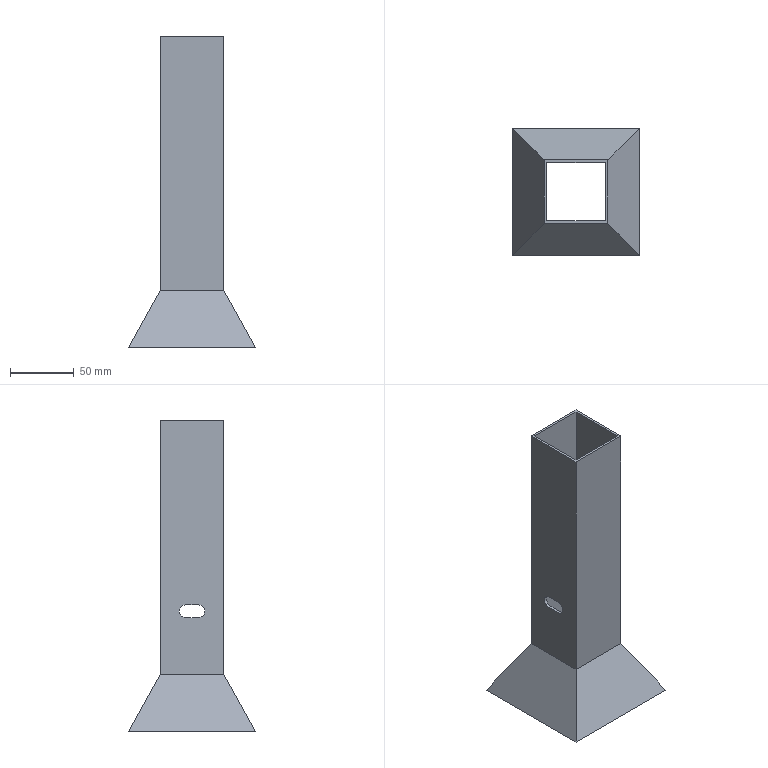Part | STEP file | Hopper | 1 solid | 28 faces | box 100 x 100 x 245 mm | volume 106017 mm3 | plane 22 | cylinder 6 | commonest cylinder face diameters 10 x6